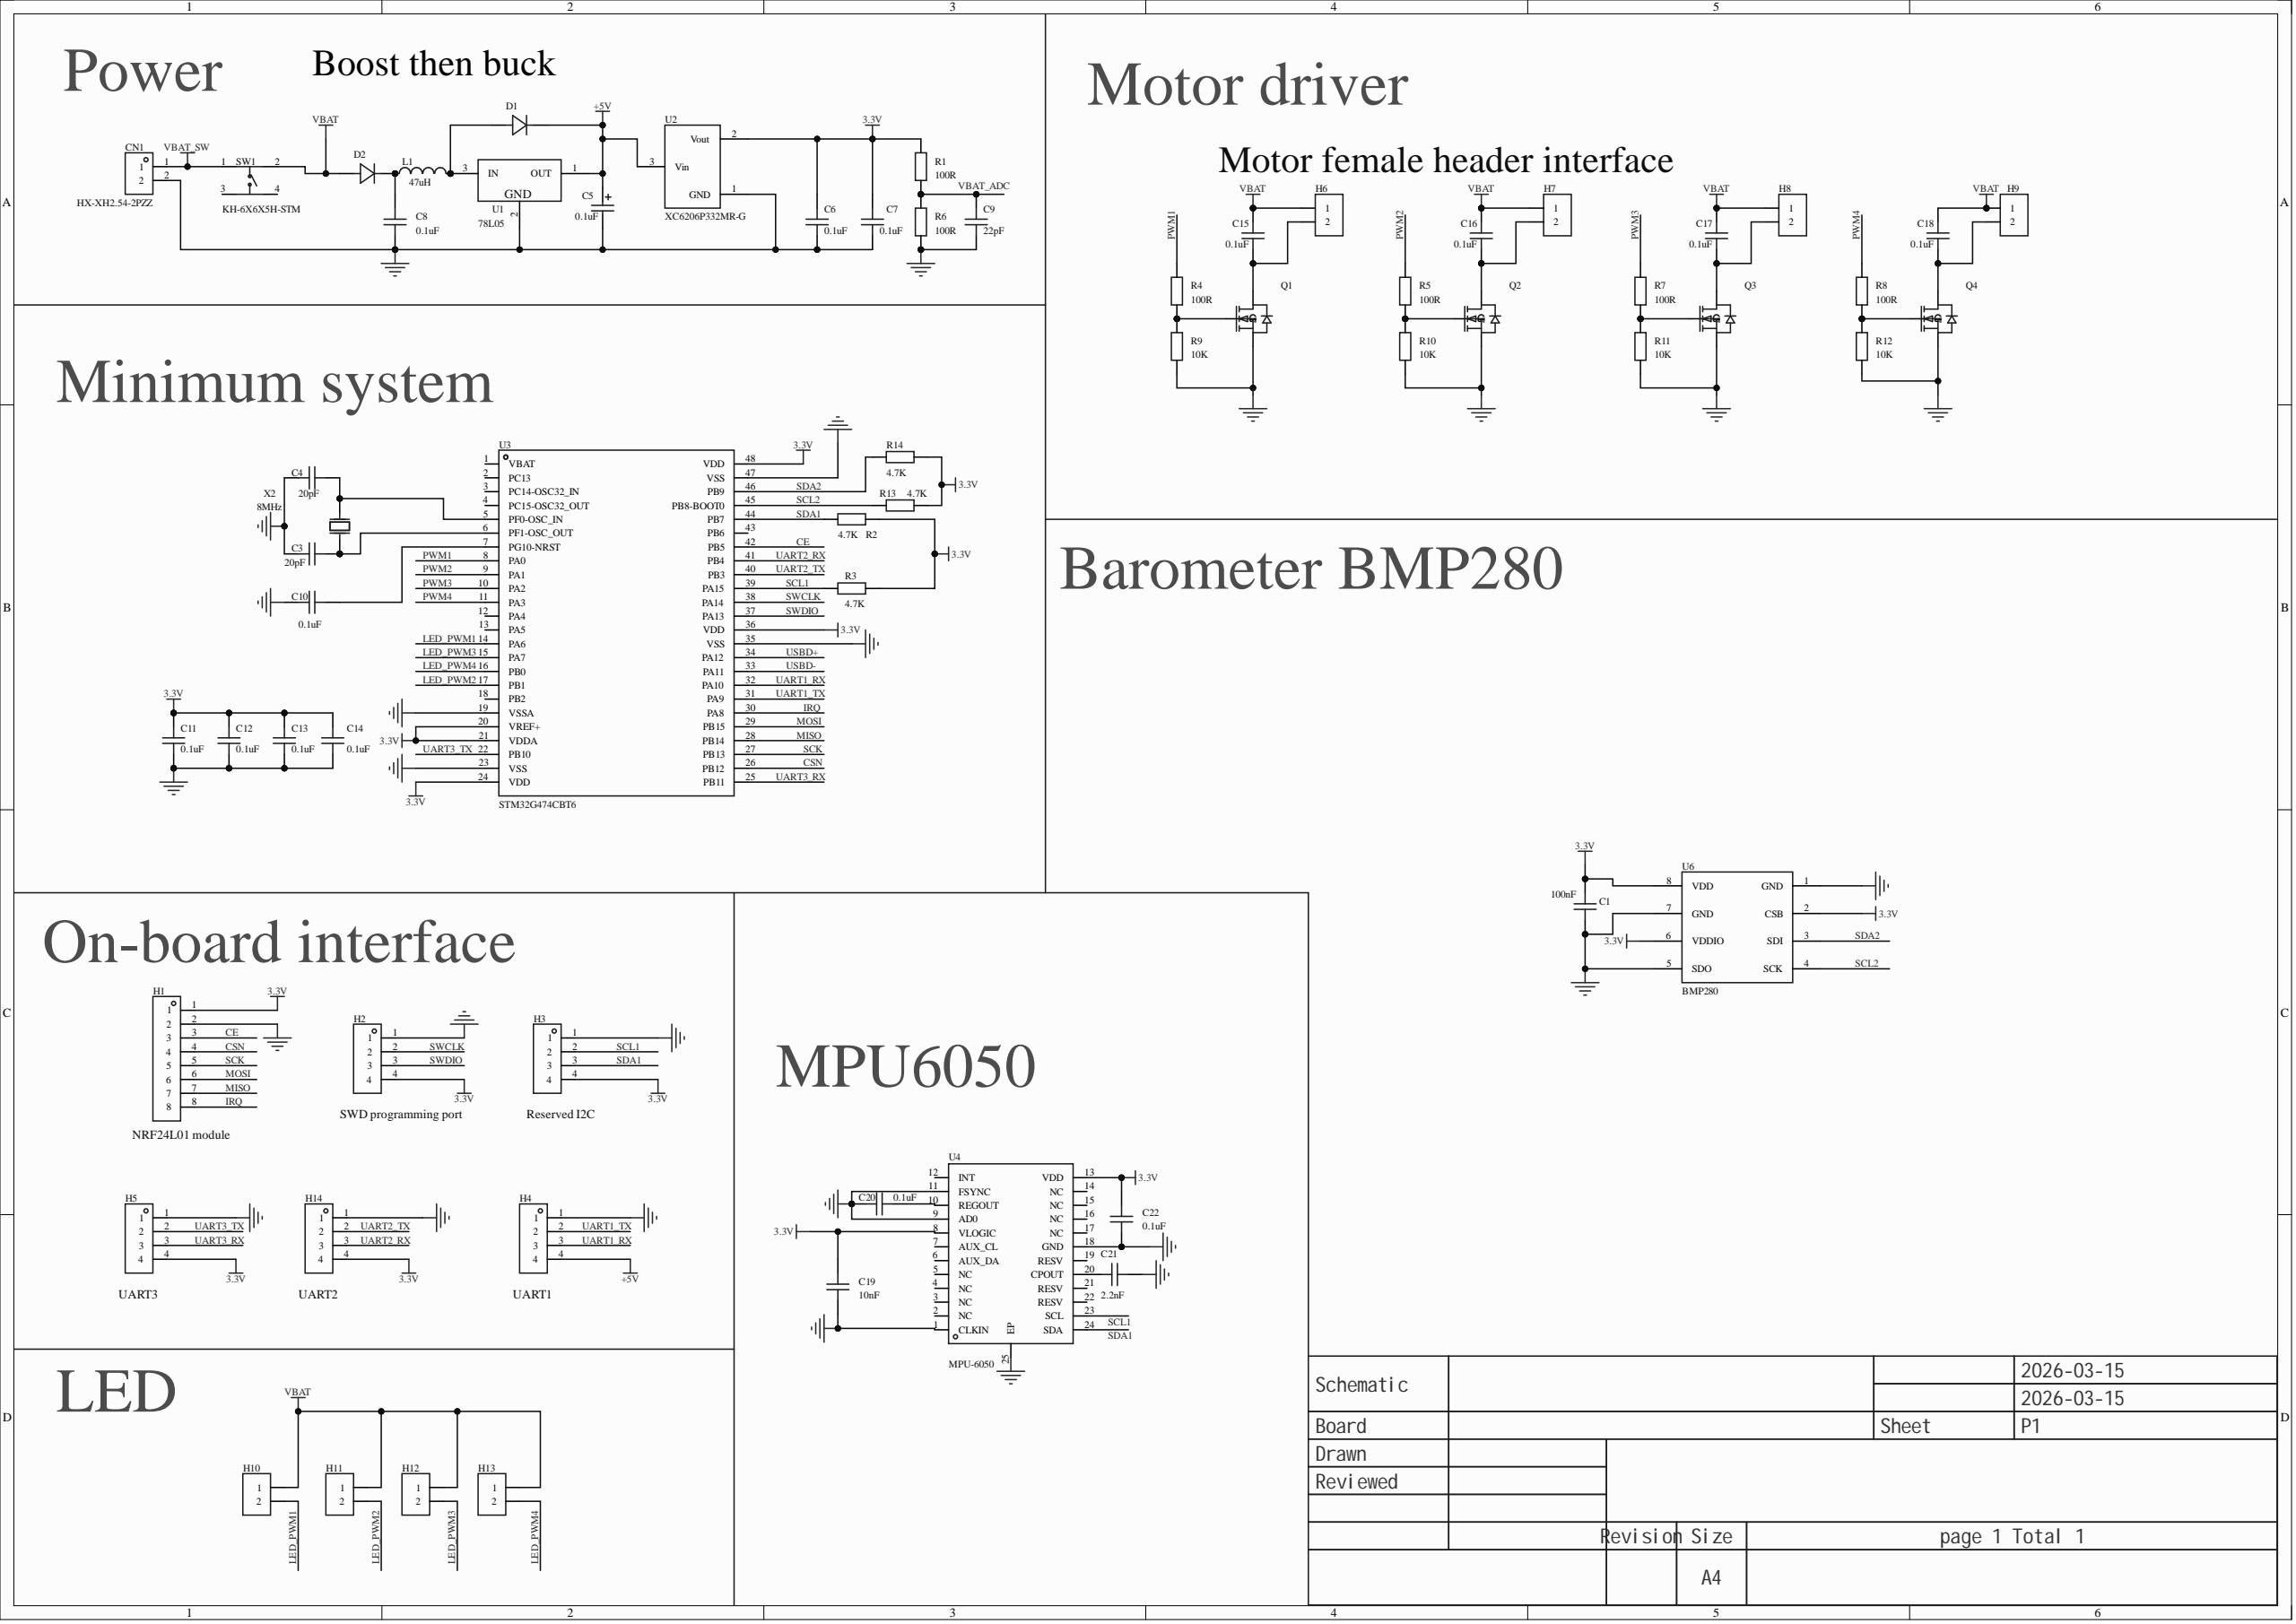Circuit board | Altium Designer | 64 parts | 47 nets
Bill of materials:
Comment,Description,Designator,Footprint,LibRef,Quantity
"100nF","","C1","C0603","CAP_0603","1"
"20pF","","C3, C4","C0603","CAP_0603","2"
"0.1uF","","C5","C_Ele_SMD_3x5.4mm","C_Ele_SMD_3x5.4mm","1"
"0.1uF","","C6, C7, C8, C10, C11, C12, C13, C14, C15, C16, C17, C18, C20, C22","C0603","CAP_0603","14"
"22pF","","C9","C0603","CAP_0603","1"
"10nF","","C19","C0603","CAP_0603","1"
"2.2nF","","C21","C0603","CAP_0603","1"
"HX-XH2.54-2PZZ","Pin structure: 1x2P; pitch: 2.54mm; mounting: through-hole; reference series: XH; total pins: 2P; rows: 1; pins per row: 2; row spacing: -; rated current: 3A; contact material: brass; contact plating: tin; operating temperature: -25℃~+85℃;","CN1","CONN-TH_2P-P2.50_HX-2.54MM-2P-ZZ-MS","HX-XH2.54-2PZZ","1"
"","","D1, D2","DO_1N4007","D_1N4007A","2"
"","","H1","HDR-TH_8P-P2.54-V-F-1","HDR-F_2.54_1x8P","1"
"","","H2, H3, H4, H5, H14","HDR-TH_4P-P2.54-V-F","HDR-F_2.54_1x4P","5"
"","","H6, H7, H8, H9, H10, H11, H12, H13","HDR-TH_2P-P2.54-V-F","HDR-F_2.54_1x2P","8"
"47uH","","L1","L0603","L_0603","1"
"","Type: N-channel; drain-source voltage (Vdss): 30V; continuous drain current (Id): 5.2A; power (Pd): 1W; on-resistance (RDS(on)@Vgs,Id): 35mO@10V,5A; threshold voltage (Vgs(th)@Id): 1.5V@250","Q1, Q2, Q3, Q4","SOT-23-3_L2.9-W1.3-P1.90-LS2.4-BR","AO3400A_N","4"
"100R","","R1, R4, R5, R6, R7, R8","R0603","Res_0603","6"
"4.7K","","R2, R3, R13, R14","R0603","Res_0603","4"
"10K","","R9, R10, R11, R12","R0603","Res_0603","4"
"KH-6X6X5H-STM","Circuit structure: SPST; button shape: round button; mounting: surface mount; switch length: 6mm; switch width: 6mm; switch height: 5mm; with bracket: without bracket; contact current: 50mA; rated voltage: 12V; service life: 8万 cycles;","SW1","SW-SMD_4P-L6.0-W6.0-P4.50-LS9.0_H5.0","KH-6X6X5H-STM","1"
"78L05","Output type: fixed; operating voltage: 30V; output voltage: 5V; output current: 100mA; ripple rejection (PSRR): 49dB@(120Hz); output polarity: positive;","U1","SOT-89-3_L4.5-W2.5-P1.50-LS4.2-BR","78L05_C347258","1"
"XC6206P332MR-G","Output type: fixed; operating voltage: 6V; output voltage: 3.3V; output current: 200mA; ripple rejection (PSRR): -; output polarity: positive;","U2","SOT-23-3_L2.9-W1.6-P1.90-LS2.8-BR","XC6206P332MR-G_C5446","1"
"STM32G474CBT6","CPU core: ARM Cortex-M4F; max CPU frequency: 170MHz; CPU bits: 32 Bit;","U3","LQFP-48_L7.0-W7.0-P0.50-LS9.0-BL","STM32G474CBT6","1"
"MPU-6050","Sensor type: accelerometer and gyroscope;","U4","QFN-24_L4.0-W4.0-P0.50-BL-EP2.7","MPU-6050","1"
"BMP280","Pressure range: 30Kpa~1.1bar; interface type: SPI; I2C;","U6","LGA-8_L2.5-W2.0-P0.65_AMP6127","BMP280","1"
"8MHz","Crystal type: SMD crystal; frequency: 8MHz; frequency tolerance at room temperature: ±10ppm; load capacitance: 20pF; frequency stability: ±20ppm;","X2","CRYSTAL-SMD_L5.0-W3.2","X50328MSB2GI","1"
Netlist (Protel format):
[
C1
C0603
100nF



]
[
C3
C0603
20pF



]
[
C4
C0603
20pF



]
[
C5
C_Ele_SMD_3x5.4mm
0.1uF



]
[
C6
C0603
0.1uF



]
[
C7
C0603
0.1uF



]
[
C8
C0603
0.1uF



]
[
C9
C0603
22pF



]
[
C10
C0603
0.1uF



]
[
C11
C0603
0.1uF



]
[
C12
C0603
0.1uF



]
[
C13
C0603
0.1uF



]
[
C14
C0603
0.1uF



]
[
C15
C0603
0.1uF



]
[
C16
C0603
0.1uF



]
[
C17
C0603
0.1uF



]
[
C18
C0603
0.1uF



]
[
C19
C0603
10nF



]
[
C20
C0603
0.1uF



]
[
C21
C0603
2.2nF



]
[
C22
C0603
0.1uF



]
[
CN1
CONN-TH_2P-P2.50_HX-2.54MM-2P-ZZ-MS
HX-XH2.54-2PZZ



]
[
D1
DO_1N4007




]
[
D2
DO_1N4007




]
[
H1
HDR-TH_8P-P2.54-V-F-1




]
[
H2
HDR-TH_4P-P2.54-V-F




]
[
H3
HDR-TH_4P-P2.54-V-F




]
[
H4
HDR-TH_4P-P2.54-V-F




]
[
H5
HDR-TH_4P-P2.54-V-F




]
[
H6
HDR-TH_2P-P2.54-V-F




]
[
H7
HDR-TH_2P-P2.54-V-F




]
[
H8
HDR-TH_2P-P2.54-V-F




]
[
H9
HDR-TH_2P-P2.54-V-F




]
[
H10
HDR-TH_2P-P2.54-V-F




]
[
H11
HDR-TH_2P-P2.54-V-F




]
[
H12
HDR-TH_2P-P2.54-V-F




]
[
H13
HDR-TH_2P-P2.54-V-F




]
[
H14
HDR-TH_4P-P2.54-V-F




]
[
L1
L0603
47uH



]
[
Q1
SOT-23-3_L2.9-W1.3-P1.90-LS2.4-BR




]
[
Q2
SOT-23-3_L2.9-W1.3-P1.90-LS2.4-BR




]
[
Q3
SOT-23-3_L2.9-W1.3-P1.90-LS2.4-BR




]
[
Q4
SOT-23-3_L2.9-W1.3-P1.90-LS2.4-BR




]
[
R1
R0603
100R



]
[
R2
R0603
4.7K



]
[
R3
R0603
4.7K



]
[
R4
R0603
100R



]
[
R5
R0603
100R



]
[
R6
R0603
100R



]
[
R7
R0603
100R



]
[
R8
R0603
100R



]
[
R9
R0603
10K



]
[
R10
R0603
10K



]
[
R11
R0603
10K



]
[
R12
R0603
10K



]
[
R13
R0603
4.7K



]
[
R14
R0603
4.7K



]
[
SW1
SW-SMD_4P-L6.0-W6.0-P4.50-LS9.0_H5.0
KH-6X6X5H-STM



]
[
U1
SOT-89-3_L4.5-W2.5-P1.50-LS4.2-BR
78L05



]
[
U2
SOT-23-3_L2.9-W1.6-P1.90-LS2.8-BR
XC6206P332MR-G



]
[
U3
LQFP-48_L7.0-W7.0-P0.50-LS9.0-BL
STM32G474CBT6



]
[
U4
QFN-24_L4.0-W4.0-P0.50-BL-EP2.7
MPU-6050



]
[
U6
LGA-8_L2.5-W2.0-P0.65_AMP6127
BMP280



]
[
X2
CRYSTAL-SMD_L5.0-W3.2
8MHz



]
(
VBAT_SW
CN1-1
SW1-1
)
(
VBAT
C15-2
C16-2
C17-2
C18-2
D2-2
H6-1
H7-1
H8-1
H9-1
H10-1
H11-1
H12-1
H13-1
SW1-2
)
(
UART3_TX
H5-2
U3-22
)
(
UART3_RX
H5-3
U3-25
)
(
UART2_TX
H14-2
U3-40
)
(
UART2_RX
H14-3
U3-41
)
(
UART1_TX
H4-2
U3-31
)
(
UART1_RX
H4-3
U3-32
)
(
SWDIO
H2-3
U3-37
)
(
SWCLK
H2-2
U3-38
)
(
SDA2
R14-1
U3-46
U6-3
)
(
SDA1
H3-3
R2-1
U3-44
U4-24
)
(
SCL2
R13-1
U3-45
U6-4
)
(
SCL1
H3-2
R3-1
U3-39
U4-23
)
(
SCK
H1-5
U3-27
)
(
PWM4
R8-2
U3-11
)
(
PWM3
R7-2
U3-10
)
(
PWM2
R5-2
U3-9
)
(
PWM1
R4-2
U3-8
)
(
NetQ4_1
Q4-1
R8-1
R12-2
)
(
NetQ3_1
Q3-1
R7-1
R11-2
)
(
NetQ2_1
Q2-1
R5-1
R10-2
)
(
NetQ1_1
Q1-1
R4-1
R9-2
)
(
NetD1_2
D1-2
L1-2
U1-3
)
(
NetC21_1
C21-1
U4-20
)
(
NetC20_2
C20-2
U4-10
)
(
NetC18_1
C18-1
H9-2
Q4-3
)
(
NetC17_1
C17-1
H8-2
Q3-3
)
(
NetC16_1
C16-1
H7-2
Q2-3
)
(
NetC15_1
C15-1
H6-2
Q1-3
)
(
NetC10_2
C10-2
U3-7
)
(
NetC9_2
C9-2
R1-1
R6-2
)
(
NetC8_2
C8-2
D2-1
L1-1
)
(
NetC4_2
C4-2
U3-5
X2-2
)
(
NetC3_2
C3-2
U3-6
X2-1
)
(
MOSI
H1-6
U3-29
)
(
MISO
H1-7
U3-28
)
(
LED_PWM4
H13-2
U3-16
)
(
LED_PWM3
H12-2
U3-15
)
(
LED_PWM2
H11-2
U3-17
)
(
LED_PWM1
H10-2
U3-14
)
(
IRQ
H1-8
U3-30
)
(
GND
C1-1
C3-1
C4-1
C5-2
C6-1
C7-1
C8-1
C9-1
C10-1
C11-1
C12-1
C13-1
C14-1
C19-1
C20-1
C21-2
C22-2
CN1-2
H1-2
H2-1
H3-1
H4-1
H5-1
H14-1
Q1-2
Q2-2
Q3-2
Q4-2
R6-1
R9-1
R10-1
R11-1
R12-1
U1-2
U2-1
U3-19
U3-23
U3-35
U3-47
U4-1
U4-9
U4-11
U4-18
U4-25
U6-1
U6-5
U6-7
)
(
CSN
H1-4
U3-26
)
(
CE
H1-3
U3-42
)
(
+5V
C5-1
D1-1
H4-4
U1-1
U2-3
)
(
3.3V
C1-2
C6-2
C7-2
C11-2
C12-2
C13-2
C14-2
C19-2
C22-1
H1-1
H2-4
H3-4
H5-4
H14-4
R1-2
R2-2
R3-2
R13-2
R14-2
U2-2
U3-20
U3-21
U3-24
U3-36
U3-48
U4-8
U4-13
U6-2
U6-6
U6-8
)